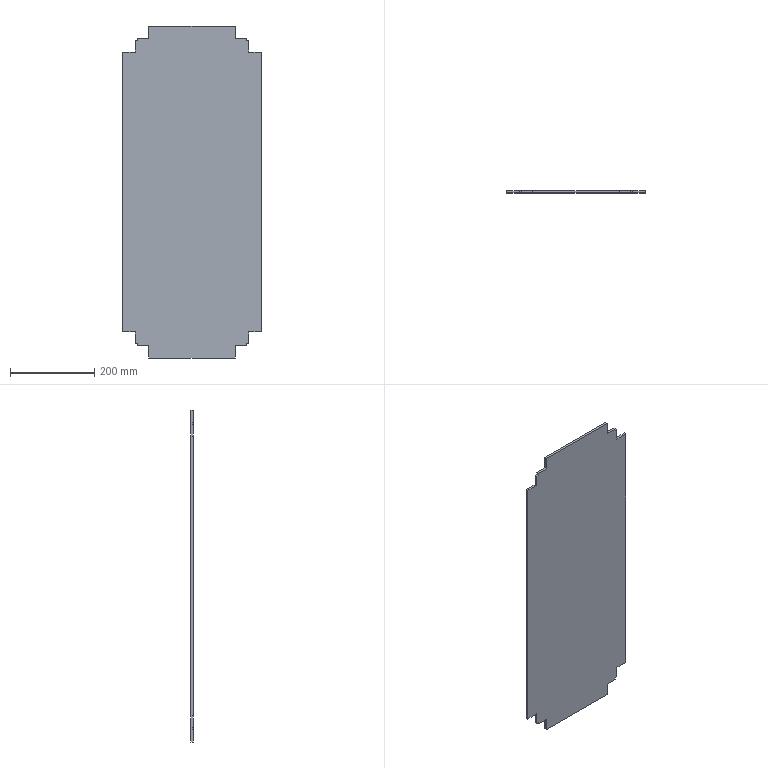Part | SolidWorks | features BaseBody 1 | 1 solid | 30 faces | box 330 x 5 x 790 mm | volume 1246600 mm3 | plane 30
STEP:
#1=CARTESIAN_POINT('',(-833.,40.,-365.));
#2=VERTEX_POINT('',#1);
#3=CARTESIAN_POINT('',(-860.,40.,-365.));
#4=VERTEX_POINT('',#3);
#5=CARTESIAN_POINT('',(-833.,40.,-365.));
#6=DIRECTION('',(-1.,0.,0.));
#7=VECTOR('',#6,1000.);
#8=LINE('',#5,#7);
#9=EDGE_CURVE('',#2,#4,#8,.T.);
#10=ORIENTED_EDGE('',*,*,#9,.F.);
#11=CARTESIAN_POINT('',(-833.,40.,-395.));
#12=VERTEX_POINT('',#11);
#13=CARTESIAN_POINT('',(-833.,40.,-395.));
#14=DIRECTION('',(0.,0.,1.));
#15=VECTOR('',#14,1000.);
#16=LINE('',#13,#15);
#17=EDGE_CURVE('',#12,#2,#16,.T.);
#18=ORIENTED_EDGE('',*,*,#17,.F.);
#19=CARTESIAN_POINT('',(-627.,40.,-395.));
#20=VERTEX_POINT('',#19);
#21=CARTESIAN_POINT('',(-627.,40.,-395.));
#22=DIRECTION('',(-1.,0.,0.));
#23=VECTOR('',#22,1000.);
#24=LINE('',#21,#23);
#25=EDGE_CURVE('',#20,#12,#24,.T.);
#26=ORIENTED_EDGE('',*,*,#25,.F.);
#27=CARTESIAN_POINT('',(-627.,40.,-365.));
#28=VERTEX_POINT('',#27);
#29=CARTESIAN_POINT('',(-627.,40.,-365.));
#30=DIRECTION('',(0.,0.,-1.));
#31=VECTOR('',#30,1000.);
#32=LINE('',#29,#31);
#33=EDGE_CURVE('',#28,#20,#32,.T.);
#34=ORIENTED_EDGE('',*,*,#33,.F.);
#35=CARTESIAN_POINT('',(-600.,40.,-365.));
#36=VERTEX_POINT('',#35);
#37=CARTESIAN_POINT('',(-600.,40.,-365.));
#38=DIRECTION('',(-1.,0.,0.));
#39=VECTOR('',#38,1000.);
#40=LINE('',#37,#39);
#41=EDGE_CURVE('',#36,#28,#40,.T.);
#42=ORIENTED_EDGE('',*,*,#41,.F.);
#43=CARTESIAN_POINT('',(-600.,40.,-360.));
#44=VERTEX_POINT('',#43);
#45=CARTESIAN_POINT('',(-600.,40.,-360.));
#46=DIRECTION('',(0.,0.,-1.));
#47=VECTOR('',#46,1000.);
#48=LINE('',#45,#47);
#49=EDGE_CURVE('',#44,#36,#48,.T.);
#50=ORIENTED_EDGE('',*,*,#49,.F.);
#51=CARTESIAN_POINT('',(-595.,40.,-360.));
#52=VERTEX_POINT('',#51);
#53=CARTESIAN_POINT('',(-595.,40.,-360.));
#54=DIRECTION('',(-1.,0.,0.));
#55=VECTOR('',#54,1000.);
#56=LINE('',#53,#55);
#57=EDGE_CURVE('',#52,#44,#56,.T.);
#58=ORIENTED_EDGE('',*,*,#57,.F.);
#59=CARTESIAN_POINT('',(-595.,40.,-333.));
#60=VERTEX_POINT('',#59);
#61=CARTESIAN_POINT('',(-595.,40.,-333.));
#62=DIRECTION('',(0.,0.,-1.));
#63=VECTOR('',#62,1000.);
#64=LINE('',#61,#63);
#65=EDGE_CURVE('',#60,#52,#64,.T.);
#66=ORIENTED_EDGE('',*,*,#65,.F.);
#67=CARTESIAN_POINT('',(-565.,40.,-333.));
#68=VERTEX_POINT('',#67);
#69=CARTESIAN_POINT('',(-565.,40.,-333.));
#70=DIRECTION('',(-1.,0.,0.));
#71=VECTOR('',#70,1000.);
#72=LINE('',#69,#71);
#73=EDGE_CURVE('',#68,#60,#72,.T.);
#74=ORIENTED_EDGE('',*,*,#73,.F.);
#75=CARTESIAN_POINT('',(-565.,40.,333.));
#76=VERTEX_POINT('',#75);
#77=CARTESIAN_POINT('',(-565.,40.,333.));
#78=DIRECTION('',(0.,0.,-1.));
#79=VECTOR('',#78,1000.);
#80=LINE('',#77,#79);
#81=EDGE_CURVE('',#76,#68,#80,.T.);
#82=ORIENTED_EDGE('',*,*,#81,.F.);
#83=CARTESIAN_POINT('',(-595.,40.,333.));
#84=VERTEX_POINT('',#83);
#85=CARTESIAN_POINT('',(-595.,40.,333.));
#86=DIRECTION('',(1.,0.,0.));
#87=VECTOR('',#86,1000.);
#88=LINE('',#85,#87);
#89=EDGE_CURVE('',#84,#76,#88,.T.);
#90=ORIENTED_EDGE('',*,*,#89,.F.);
#91=CARTESIAN_POINT('',(-595.,40.,360.));
#92=VERTEX_POINT('',#91);
#93=CARTESIAN_POINT('',(-595.,40.,360.));
#94=DIRECTION('',(0.,0.,-1.));
#95=VECTOR('',#94,1000.);
#96=LINE('',#93,#95);
#97=EDGE_CURVE('',#92,#84,#96,.T.);
#98=ORIENTED_EDGE('',*,*,#97,.F.);
#99=CARTESIAN_POINT('',(-600.,40.,360.));
#100=VERTEX_POINT('',#99);
#101=CARTESIAN_POINT('',(-600.,40.,360.));
#102=DIRECTION('',(1.,0.,0.));
#103=VECTOR('',#102,1000.);
#104=LINE('',#101,#103);
#105=EDGE_CURVE('',#100,#92,#104,.T.);
#106=ORIENTED_EDGE('',*,*,#105,.F.);
#107=CARTESIAN_POINT('',(-600.,40.,365.));
#108=VERTEX_POINT('',#107);
#109=CARTESIAN_POINT('',(-600.,40.,365.));
#110=DIRECTION('',(0.,0.,-1.));
#111=VECTOR('',#110,1000.);
#112=LINE('',#109,#111);
#113=EDGE_CURVE('',#108,#100,#112,.T.);
#114=ORIENTED_EDGE('',*,*,#113,.F.);
#115=CARTESIAN_POINT('',(-627.,40.,365.));
#116=VERTEX_POINT('',#115);
#117=CARTESIAN_POINT('',(-627.,40.,365.));
#118=DIRECTION('',(1.,0.,0.));
#119=VECTOR('',#118,1000.);
#120=LINE('',#117,#119);
#121=EDGE_CURVE('',#116,#108,#120,.T.);
#122=ORIENTED_EDGE('',*,*,#121,.F.);
#123=CARTESIAN_POINT('',(-627.,40.,395.));
#124=VERTEX_POINT('',#123);
#125=CARTESIAN_POINT('',(-627.,40.,395.));
#126=DIRECTION('',(0.,0.,-1.));
#127=VECTOR('',#126,1000.);
#128=LINE('',#125,#127);
#129=EDGE_CURVE('',#124,#116,#128,.T.);
#130=ORIENTED_EDGE('',*,*,#129,.F.);
#131=CARTESIAN_POINT('',(-833.,40.,395.));
#132=VERTEX_POINT('',#131);
#133=CARTESIAN_POINT('',(-833.,40.,395.));
#134=DIRECTION('',(1.,0.,0.));
#135=VECTOR('',#134,1000.);
#136=LINE('',#133,#135);
#137=EDGE_CURVE('',#132,#124,#136,.T.);
#138=ORIENTED_EDGE('',*,*,#137,.F.);
#139=CARTESIAN_POINT('',(-833.,40.,365.));
#140=VERTEX_POINT('',#139);
#141=CARTESIAN_POINT('',(-833.,40.,365.));
#142=DIRECTION('',(0.,0.,1.));
#143=VECTOR('',#142,1000.);
#144=LINE('',#141,#143);
#145=EDGE_CURVE('',#140,#132,#144,.T.);
#146=ORIENTED_EDGE('',*,*,#145,.F.);
#147=CARTESIAN_POINT('',(-860.,40.,365.));
#148=VERTEX_POINT('',#147);
#149=CARTESIAN_POINT('',(-860.,40.,365.));
#150=DIRECTION('',(1.,0.,0.));
#151=VECTOR('',#150,1000.);
#152=LINE('',#149,#151);
#153=EDGE_CURVE('',#148,#140,#152,.T.);
#154=ORIENTED_EDGE('',*,*,#153,.F.);
#155=CARTESIAN_POINT('',(-860.,40.,360.));
#156=VERTEX_POINT('',#155);
#157=CARTESIAN_POINT('',(-860.,40.,360.));
#158=DIRECTION('',(0.,0.,1.));
#159=VECTOR('',#158,1000.);
#160=LINE('',#157,#159);
#161=EDGE_CURVE('',#156,#148,#160,.T.);
#162=ORIENTED_EDGE('',*,*,#161,.F.);
#163=CARTESIAN_POINT('',(-865.,40.,360.));
#164=VERTEX_POINT('',#163);
#165=CARTESIAN_POINT('',(-865.,40.,360.));
#166=DIRECTION('',(1.,0.,0.));
#167=VECTOR('',#166,1000.);
#168=LINE('',#165,#167);
#169=EDGE_CURVE('',#164,#156,#168,.T.);
#170=ORIENTED_EDGE('',*,*,#169,.F.);
#171=CARTESIAN_POINT('',(-865.,40.,333.));
#172=VERTEX_POINT('',#171);
#173=CARTESIAN_POINT('',(-865.,40.,333.));
#174=DIRECTION('',(0.,0.,1.));
#175=VECTOR('',#174,1000.);
#176=LINE('',#173,#175);
#177=EDGE_CURVE('',#172,#164,#176,.T.);
#178=ORIENTED_EDGE('',*,*,#177,.F.);
#179=CARTESIAN_POINT('',(-895.,40.,333.));
#180=VERTEX_POINT('',#179);
#181=CARTESIAN_POINT('',(-895.,40.,333.));
#182=DIRECTION('',(1.,0.,0.));
#183=VECTOR('',#182,1000.);
#184=LINE('',#181,#183);
#185=EDGE_CURVE('',#180,#172,#184,.T.);
#186=ORIENTED_EDGE('',*,*,#185,.F.);
#187=CARTESIAN_POINT('',(-895.,40.,-333.));
#188=VERTEX_POINT('',#187);
#189=CARTESIAN_POINT('',(-895.,40.,-333.));
#190=DIRECTION('',(0.,0.,1.));
#191=VECTOR('',#190,1000.);
#192=LINE('',#189,#191);
#193=EDGE_CURVE('',#188,#180,#192,.T.);
#194=ORIENTED_EDGE('',*,*,#193,.F.);
#195=CARTESIAN_POINT('',(-865.,40.,-333.));
#196=VERTEX_POINT('',#195);
#197=CARTESIAN_POINT('',(-865.,40.,-333.));
#198=DIRECTION('',(-1.,0.,0.));
#199=VECTOR('',#198,1000.);
#200=LINE('',#197,#199);
#201=EDGE_CURVE('',#196,#188,#200,.T.);
#202=ORIENTED_EDGE('',*,*,#201,.F.);
#203=CARTESIAN_POINT('',(-865.,40.,-360.));
#204=VERTEX_POINT('',#203);
#205=CARTESIAN_POINT('',(-865.,40.,-360.));
#206=DIRECTION('',(0.,0.,1.));
#207=VECTOR('',#206,1000.);
#208=LINE('',#205,#207);
#209=EDGE_CURVE('',#204,#196,#208,.T.);
#210=ORIENTED_EDGE('',*,*,#209,.F.);
#211=CARTESIAN_POINT('',(-860.,40.,-360.));
#212=VERTEX_POINT('',#211);
#213=CARTESIAN_POINT('',(-860.,40.,-360.));
#214=DIRECTION('',(-1.,0.,0.));
#215=VECTOR('',#214,1000.);
#216=LINE('',#213,#215);
#217=EDGE_CURVE('',#212,#204,#216,.T.);
#218=ORIENTED_EDGE('',*,*,#217,.F.);
#219=CARTESIAN_POINT('',(-860.,40.,-365.));
#220=DIRECTION('',(0.,0.,1.));
#221=VECTOR('',#220,1000.);
#222=LINE('',#219,#221);
#223=EDGE_CURVE('',#4,#212,#222,.T.);
#224=ORIENTED_EDGE('',*,*,#223,.F.);
#225=EDGE_LOOP('',(#10,#18,#26,#34,#42,#50,#58,#66,#74,#82,#90,#98,#106,#114,#122,#130,#138,#146,#154,#162,#170,#178,#186,#194,#202,#210,#218,#224));
#226=FACE_OUTER_BOUND('',#225,.T.);
#227=CARTESIAN_POINT('',(-730.,40.,0.));
#228=DIRECTION('',(0.,-1.,0.));
#229=DIRECTION('',(0.,0.,-1.));
#230=AXIS2_PLACEMENT_3D('',#227,#228,#229);
#231=PLANE('',#230);
#232=ADVANCED_FACE('',(#226),#231,.T.);
#233=CARTESIAN_POINT('',(-860.,45.,-365.));
#234=VERTEX_POINT('',#233);
#235=CARTESIAN_POINT('',(-833.,45.,-365.));
#236=VERTEX_POINT('',#235);
#237=CARTESIAN_POINT('',(-860.,45.,-365.));
#238=DIRECTION('',(1.,0.,0.));
#239=VECTOR('',#238,1000.);
#240=LINE('',#237,#239);
#241=EDGE_CURVE('',#234,#236,#240,.T.);
#242=ORIENTED_EDGE('',*,*,#241,.F.);
#243=CARTESIAN_POINT('',(-860.,45.,-360.));
#244=VERTEX_POINT('',#243);
#245=CARTESIAN_POINT('',(-860.,45.,-360.));
#246=DIRECTION('',(0.,0.,-1.));
#247=VECTOR('',#246,1000.);
#248=LINE('',#245,#247);
#249=EDGE_CURVE('',#244,#234,#248,.T.);
#250=ORIENTED_EDGE('',*,*,#249,.F.);
#251=CARTESIAN_POINT('',(-865.,45.,-360.));
#252=VERTEX_POINT('',#251);
#253=CARTESIAN_POINT('',(-865.,45.,-360.));
#254=DIRECTION('',(1.,0.,0.));
#255=VECTOR('',#254,1000.);
#256=LINE('',#253,#255);
#257=EDGE_CURVE('',#252,#244,#256,.T.);
#258=ORIENTED_EDGE('',*,*,#257,.F.);
#259=CARTESIAN_POINT('',(-865.,45.,-333.));
#260=VERTEX_POINT('',#259);
#261=CARTESIAN_POINT('',(-865.,45.,-333.));
#262=DIRECTION('',(0.,0.,-1.));
#263=VECTOR('',#262,1000.);
#264=LINE('',#261,#263);
#265=EDGE_CURVE('',#260,#252,#264,.T.);
#266=ORIENTED_EDGE('',*,*,#265,.F.);
#267=CARTESIAN_POINT('',(-895.,45.,-333.));
#268=VERTEX_POINT('',#267);
#269=CARTESIAN_POINT('',(-895.,45.,-333.));
#270=DIRECTION('',(1.,0.,0.));
#271=VECTOR('',#270,1000.);
#272=LINE('',#269,#271);
#273=EDGE_CURVE('',#268,#260,#272,.T.);
#274=ORIENTED_EDGE('',*,*,#273,.F.);
#275=CARTESIAN_POINT('',(-895.,45.,333.));
#276=VERTEX_POINT('',#275);
#277=CARTESIAN_POINT('',(-895.,45.,333.));
#278=DIRECTION('',(0.,0.,-1.));
#279=VECTOR('',#278,1000.);
#280=LINE('',#277,#279);
#281=EDGE_CURVE('',#276,#268,#280,.T.);
#282=ORIENTED_EDGE('',*,*,#281,.F.);
#283=CARTESIAN_POINT('',(-865.,45.,333.));
#284=VERTEX_POINT('',#283);
#285=CARTESIAN_POINT('',(-865.,45.,333.));
#286=DIRECTION('',(-1.,0.,0.));
#287=VECTOR('',#286,1000.);
#288=LINE('',#285,#287);
#289=EDGE_CURVE('',#284,#276,#288,.T.);
#290=ORIENTED_EDGE('',*,*,#289,.F.);
#291=CARTESIAN_POINT('',(-865.,45.,360.));
#292=VERTEX_POINT('',#291);
#293=CARTESIAN_POINT('',(-865.,45.,360.));
#294=DIRECTION('',(0.,0.,-1.));
#295=VECTOR('',#294,1000.);
#296=LINE('',#293,#295);
#297=EDGE_CURVE('',#292,#284,#296,.T.);
#298=ORIENTED_EDGE('',*,*,#297,.F.);
#299=CARTESIAN_POINT('',(-860.,45.,360.));
#300=VERTEX_POINT('',#299);
#301=CARTESIAN_POINT('',(-860.,45.,360.));
#302=DIRECTION('',(-1.,0.,0.));
#303=VECTOR('',#302,1000.);
#304=LINE('',#301,#303);
#305=EDGE_CURVE('',#300,#292,#304,.T.);
#306=ORIENTED_EDGE('',*,*,#305,.F.);
#307=CARTESIAN_POINT('',(-860.,45.,365.));
#308=VERTEX_POINT('',#307);
#309=CARTESIAN_POINT('',(-860.,45.,365.));
#310=DIRECTION('',(0.,0.,-1.));
#311=VECTOR('',#310,1000.);
#312=LINE('',#309,#311);
#313=EDGE_CURVE('',#308,#300,#312,.T.);
#314=ORIENTED_EDGE('',*,*,#313,.F.);
#315=CARTESIAN_POINT('',(-833.,45.,365.));
#316=VERTEX_POINT('',#315);
#317=CARTESIAN_POINT('',(-833.,45.,365.));
#318=DIRECTION('',(-1.,0.,0.));
#319=VECTOR('',#318,1000.);
#320=LINE('',#317,#319);
#321=EDGE_CURVE('',#316,#308,#320,.T.);
#322=ORIENTED_EDGE('',*,*,#321,.F.);
#323=CARTESIAN_POINT('',(-833.,45.,395.));
#324=VERTEX_POINT('',#323);
#325=CARTESIAN_POINT('',(-833.,45.,395.));
#326=DIRECTION('',(0.,0.,-1.));
#327=VECTOR('',#326,1000.);
#328=LINE('',#325,#327);
#329=EDGE_CURVE('',#324,#316,#328,.T.);
#330=ORIENTED_EDGE('',*,*,#329,.F.);
#331=CARTESIAN_POINT('',(-627.,45.,395.));
#332=VERTEX_POINT('',#331);
#333=CARTESIAN_POINT('',(-627.,45.,395.));
#334=DIRECTION('',(-1.,0.,0.));
#335=VECTOR('',#334,1000.);
#336=LINE('',#333,#335);
#337=EDGE_CURVE('',#332,#324,#336,.T.);
#338=ORIENTED_EDGE('',*,*,#337,.F.);
#339=CARTESIAN_POINT('',(-627.,45.,365.));
#340=VERTEX_POINT('',#339);
#341=CARTESIAN_POINT('',(-627.,45.,365.));
#342=DIRECTION('',(0.,0.,1.));
#343=VECTOR('',#342,1000.);
#344=LINE('',#341,#343);
#345=EDGE_CURVE('',#340,#332,#344,.T.);
#346=ORIENTED_EDGE('',*,*,#345,.F.);
#347=CARTESIAN_POINT('',(-600.,45.,365.));
#348=VERTEX_POINT('',#347);
#349=CARTESIAN_POINT('',(-600.,45.,365.));
#350=DIRECTION('',(-1.,0.,0.));
#351=VECTOR('',#350,1000.);
#352=LINE('',#349,#351);
#353=EDGE_CURVE('',#348,#340,#352,.T.);
#354=ORIENTED_EDGE('',*,*,#353,.F.);
#355=CARTESIAN_POINT('',(-600.,45.,360.));
#356=VERTEX_POINT('',#355);
#357=CARTESIAN_POINT('',(-600.,45.,360.));
#358=DIRECTION('',(0.,0.,1.));
#359=VECTOR('',#358,1000.);
#360=LINE('',#357,#359);
#361=EDGE_CURVE('',#356,#348,#360,.T.);
#362=ORIENTED_EDGE('',*,*,#361,.F.);
#363=CARTESIAN_POINT('',(-595.,45.,360.));
#364=VERTEX_POINT('',#363);
#365=CARTESIAN_POINT('',(-595.,45.,360.));
#366=DIRECTION('',(-1.,0.,0.));
#367=VECTOR('',#366,1000.);
#368=LINE('',#365,#367);
#369=EDGE_CURVE('',#364,#356,#368,.T.);
#370=ORIENTED_EDGE('',*,*,#369,.F.);
#371=CARTESIAN_POINT('',(-595.,45.,333.));
#372=VERTEX_POINT('',#371);
#373=CARTESIAN_POINT('',(-595.,45.,333.));
#374=DIRECTION('',(0.,0.,1.));
#375=VECTOR('',#374,1000.);
#376=LINE('',#373,#375);
#377=EDGE_CURVE('',#372,#364,#376,.T.);
#378=ORIENTED_EDGE('',*,*,#377,.F.);
#379=CARTESIAN_POINT('',(-565.,45.,333.));
#380=VERTEX_POINT('',#379);
#381=CARTESIAN_POINT('',(-565.,45.,333.));
#382=DIRECTION('',(-1.,0.,0.));
#383=VECTOR('',#382,1000.);
#384=LINE('',#381,#383);
#385=EDGE_CURVE('',#380,#372,#384,.T.);
#386=ORIENTED_EDGE('',*,*,#385,.F.);
#387=CARTESIAN_POINT('',(-565.,45.,-333.));
#388=VERTEX_POINT('',#387);
#389=CARTESIAN_POINT('',(-565.,45.,-333.));
#390=DIRECTION('',(0.,0.,1.));
#391=VECTOR('',#390,1000.);
#392=LINE('',#389,#391);
#393=EDGE_CURVE('',#388,#380,#392,.T.);
#394=ORIENTED_EDGE('',*,*,#393,.F.);
#395=CARTESIAN_POINT('',(-595.,45.,-333.));
#396=VERTEX_POINT('',#395);
#397=CARTESIAN_POINT('',(-595.,45.,-333.));
#398=DIRECTION('',(1.,0.,0.));
#399=VECTOR('',#398,1000.);
#400=LINE('',#397,#399);
#401=EDGE_CURVE('',#396,#388,#400,.T.);
#402=ORIENTED_EDGE('',*,*,#401,.F.);
#403=CARTESIAN_POINT('',(-595.,45.,-360.));
#404=VERTEX_POINT('',#403);
#405=CARTESIAN_POINT('',(-595.,45.,-360.));
#406=DIRECTION('',(0.,0.,1.));
#407=VECTOR('',#406,1000.);
#408=LINE('',#405,#407);
#409=EDGE_CURVE('',#404,#396,#408,.T.);
#410=ORIENTED_EDGE('',*,*,#409,.F.);
#411=CARTESIAN_POINT('',(-600.,45.,-360.));
#412=VERTEX_POINT('',#411);
#413=CARTESIAN_POINT('',(-600.,45.,-360.));
#414=DIRECTION('',(1.,0.,0.));
#415=VECTOR('',#414,1000.);
#416=LINE('',#413,#415);
#417=EDGE_CURVE('',#412,#404,#416,.T.);
#418=ORIENTED_EDGE('',*,*,#417,.F.);
#419=CARTESIAN_POINT('',(-600.,45.,-365.));
#420=VERTEX_POINT('',#419);
#421=CARTESIAN_POINT('',(-600.,45.,-365.));
#422=DIRECTION('',(0.,0.,1.));
#423=VECTOR('',#422,1000.);
#424=LINE('',#421,#423);
#425=EDGE_CURVE('',#420,#412,#424,.T.);
#426=ORIENTED_EDGE('',*,*,#425,.F.);
#427=CARTESIAN_POINT('',(-627.,45.,-365.));
#428=VERTEX_POINT('',#427);
#429=CARTESIAN_POINT('',(-627.,45.,-365.));
#430=DIRECTION('',(1.,0.,0.));
#431=VECTOR('',#430,1000.);
#432=LINE('',#429,#431);
#433=EDGE_CURVE('',#428,#420,#432,.T.);
#434=ORIENTED_EDGE('',*,*,#433,.F.);
#435=CARTESIAN_POINT('',(-627.,45.,-395.));
#436=VERTEX_POINT('',#435);
#437=CARTESIAN_POINT('',(-627.,45.,-395.));
#438=DIRECTION('',(0.,0.,1.));
#439=VECTOR('',#438,1000.);
#440=LINE('',#437,#439);
#441=EDGE_CURVE('',#436,#428,#440,.T.);
#442=ORIENTED_EDGE('',*,*,#441,.F.);
#443=CARTESIAN_POINT('',(-833.,45.,-395.));
#444=VERTEX_POINT('',#443);
#445=CARTESIAN_POINT('',(-833.,45.,-395.));
#446=DIRECTION('',(1.,0.,0.));
#447=VECTOR('',#446,1000.);
#448=LINE('',#445,#447);
#449=EDGE_CURVE('',#444,#436,#448,.T.);
#450=ORIENTED_EDGE('',*,*,#449,.F.);
#451=CARTESIAN_POINT('',(-833.,45.,-365.));
#452=DIRECTION('',(0.,0.,-1.));
#453=VECTOR('',#452,1000.);
#454=LINE('',#451,#453);
#455=EDGE_CURVE('',#236,#444,#454,.T.);
#456=ORIENTED_EDGE('',*,*,#455,.F.);
#457=EDGE_LOOP('',(#242,#250,#258,#266,#274,#282,#290,#298,#306,#314,#322,#330,#338,#346,#354,#362,#370,#378,#386,#394,#402,#410,#418,#426,#434,#442,#450,#456));
#458=FACE_OUTER_BOUND('',#457,.T.);
#459=CARTESIAN_POINT('',(-730.,45.,0.));
#460=DIRECTION('',(0.,1.,0.));
#461=DIRECTION('',(1.,0.,0.));
#462=AXIS2_PLACEMENT_3D('',#459,#460,#461);
#463=PLANE('',#462);
#464=ADVANCED_FACE('',(#458),#463,.T.);
#465=ORIENTED_EDGE('',*,*,#9,.T.);
#466=CARTESIAN_POINT('',(-860.,45.,-365.));
#467=DIRECTION('',(0.,-1.,0.));
#468=VECTOR('',#467,1000.);
#469=LINE('',#466,#468);
#470=EDGE_CURVE('',#234,#4,#469,.T.);
#471=ORIENTED_EDGE('',*,*,#470,.F.);
#472=ORIENTED_EDGE('',*,*,#241,.T.);
#473=CARTESIAN_POINT('',(-833.,40.,-365.));
#474=DIRECTION('',(0.,1.,0.));
#475=VECTOR('',#474,1000.);
#476=LINE('',#473,#475);
#477=EDGE_CURVE('',#2,#236,#476,.T.);
#478=ORIENTED_EDGE('',*,*,#477,.F.);
#479=EDGE_LOOP('',(#465,#471,#472,#478));
#480=FACE_OUTER_BOUND('',#479,.T.);
#481=CARTESIAN_POINT('',(-833.,40.,-365.));
#482=DIRECTION('',(0.,0.,-1.));
#483=DIRECTION('',(0.,-1.,0.));
#484=AXIS2_PLACEMENT_3D('',#481,#482,#483);
#485=PLANE('',#484);
#486=ADVANCED_FACE('',(#480),#485,.T.);
#487=ORIENTED_EDGE('',*,*,#223,.T.);
#488=CARTESIAN_POINT('',(-860.,45.,-360.));
#489=DIRECTION('',(0.,-1.,0.));
#490=VECTOR('',#489,1000.);
#491=LINE('',#488,#490);
#492=EDGE_CURVE('',#244,#212,#491,.T.);
#493=ORIENTED_EDGE('',*,*,#492,.F.);
#494=ORIENTED_EDGE('',*,*,#249,.T.);
#495=ORIENTED_EDGE('',*,*,#470,.T.);
#496=EDGE_LOOP('',(#487,#493,#494,#495));
#497=FACE_OUTER_BOUND('',#496,.T.);
#498=CARTESIAN_POINT('',(-860.,40.,-365.));
#499=DIRECTION('',(-1.,0.,0.));
#500=DIRECTION('',(0.,0.,1.));
#501=AXIS2_PLACEMENT_3D('',#498,#499,#500);
#502=PLANE('',#501);
#503=ADVANCED_FACE('',(#497),#502,.T.);
#504=ORIENTED_EDGE('',*,*,#217,.T.);
#505=CARTESIAN_POINT('',(-865.,45.,-360.));
#506=DIRECTION('',(0.,-1.,0.));
#507=VECTOR('',#506,1000.);
#508=LINE('',#505,#507);
#509=EDGE_CURVE('',#252,#204,#508,.T.);
#510=ORIENTED_EDGE('',*,*,#509,.F.);
#511=ORIENTED_EDGE('',*,*,#257,.T.);
#512=ORIENTED_EDGE('',*,*,#492,.T.);
#513=EDGE_LOOP('',(#504,#510,#511,#512));
#514=FACE_OUTER_BOUND('',#513,.T.);
#515=CARTESIAN_POINT('',(-860.,40.,-360.));
#516=DIRECTION('',(0.,0.,-1.));
#517=DIRECTION('',(0.,-1.,0.));
#518=AXIS2_PLACEMENT_3D('',#515,#516,#517);
#519=PLANE('',#518);
#520=ADVANCED_FACE('',(#514),#519,.T.);
#521=ORIENTED_EDGE('',*,*,#209,.T.);
#522=CARTESIAN_POINT('',(-865.,45.,-333.));
#523=DIRECTION('',(0.,-1.,0.));
#524=VECTOR('',#523,1000.);
#525=LINE('',#522,#524);
#526=EDGE_CURVE('',#260,#196,#525,.T.);
#527=ORIENTED_EDGE('',*,*,#526,.F.);
#528=ORIENTED_EDGE('',*,*,#265,.T.);
#529=ORIENTED_EDGE('',*,*,#509,.T.);
#530=EDGE_LOOP('',(#521,#527,#528,#529));
#531=FACE_OUTER_BOUND('',#530,.T.);
#532=CARTESIAN_POINT('',(-865.,40.,-360.));
#533=DIRECTION('',(-1.,0.,0.));
#534=DIRECTION('',(0.,0.,1.));
#535=AXIS2_PLACEMENT_3D('',#532,#533,#534);
#536=PLANE('',#535);
#537=ADVANCED_FACE('',(#531),#536,.T.);
#538=ORIENTED_EDGE('',*,*,#201,.T.);
#539=CARTESIAN_POINT('',(-895.,45.,-333.));
#540=DIRECTION('',(0.,-1.,0.));
#541=VECTOR('',#540,1000.);
#542=LINE('',#539,#541);
#543=EDGE_CURVE('',#268,#188,#542,.T.);
#544=ORIENTED_EDGE('',*,*,#543,.F.);
#545=ORIENTED_EDGE('',*,*,#273,.T.);
#546=ORIENTED_EDGE('',*,*,#526,.T.);
#547=EDGE_LOOP('',(#538,#544,#545,#546));
#548=FACE_OUTER_BOUND('',#547,.T.);
#549=CARTESIAN_POINT('',(-865.,40.,-333.));
#550=DIRECTION('',(0.,0.,-1.));
#551=DIRECTION('',(0.,-1.,0.));
#552=AXIS2_PLACEMENT_3D('',#549,#550,#551);
#553=PLANE('',#552);
#554=ADVANCED_FACE('',(#548),#553,.T.);
#555=ORIENTED_EDGE('',*,*,#193,.T.);
#556=CARTESIAN_POINT('',(-895.,45.,333.));
#557=DIRECTION('',(0.,-1.,0.));
#558=VECTOR('',#557,1000.);
#559=LINE('',#556,#558);
#560=EDGE_CURVE('',#276,#180,#559,.T.);
#561=ORIENTED_EDGE('',*,*,#560,.F.);
#562=ORIENTED_EDGE('',*,*,#281,.T.);
#563=ORIENTED_EDGE('',*,*,#543,.T.);
#564=EDGE_LOOP('',(#555,#561,#562,#563));
#565=FACE_OUTER_BOUND('',#564,.T.);
#566=CARTESIAN_POINT('',(-895.,40.,-333.));
#567=DIRECTION('',(-1.,0.,0.));
#568=DIRECTION('',(0.,0.,1.));
#569=AXIS2_PLACEMENT_3D('',#566,#567,#568);
#570=PLANE('',#569);
#571=ADVANCED_FACE('',(#565),#570,.T.);
#572=ORIENTED_EDGE('',*,*,#185,.T.);
#573=CARTESIAN_POINT('',(-865.,45.,333.));
#574=DIRECTION('',(0.,-1.,0.));
#575=VECTOR('',#574,1000.);
#576=LINE('',#573,#575);
#577=EDGE_CURVE('',#284,#172,#576,.T.);
#578=ORIENTED_EDGE('',*,*,#577,.F.);
#579=ORIENTED_EDGE('',*,*,#289,.T.);
#580=ORIENTED_EDGE('',*,*,#560,.T.);
#581=EDGE_LOOP('',(#572,#578,#579,#580));
#582=FACE_OUTER_BOUND('',#581,.T.);
#583=CARTESIAN_POINT('',(-895.,40.,333.));
#584=DIRECTION('',(0.,0.,1.));
#585=DIRECTION('',(1.,0.,0.));
#586=AXIS2_PLACEMENT_3D('',#583,#584,#585);
#587=PLANE('',#586);
#588=ADVANCED_FACE('',(#582),#587,.T.);
#589=ORIENTED_EDGE('',*,*,#177,.T.);
#590=CARTESIAN_POINT('',(-865.,45.,360.));
#591=DIRECTION('',(0.,-1.,0.));
#592=VECTOR('',#591,1000.);
#593=LINE('',#590,#592);
#594=EDGE_CURVE('',#292,#164,#593,.T.);
#595=ORIENTED_EDGE('',*,*,#594,.F.);
#596=ORIENTED_EDGE('',*,*,#297,.T.);
#597=ORIENTED_EDGE('',*,*,#577,.T.);
#598=EDGE_LOOP('',(#589,#595,#596,#597));
#599=FACE_OUTER_BOUND('',#598,.T.);
#600=CARTESIAN_POINT('',(-865.,40.,333.));
#601=DIRECTION('',(-1.,0.,0.));
#602=DIRECTION('',(0.,0.,1.));
#603=AXIS2_PLACEMENT_3D('',#600,#601,#602);
#604=PLANE('',#603);
#605=ADVANCED_FACE('',(#599),#604,.T.);
#606=ORIENTED_EDGE('',*,*,#169,.T.);
#607=CARTESIAN_POINT('',(-860.,45.,360.));
#608=DIRECTION('',(0.,-1.,0.));
#609=VECTOR('',#608,1000.);
#610=LINE('',#607,#609);
#611=EDGE_CURVE('',#300,#156,#610,.T.);
#612=ORIENTED_EDGE('',*,*,#611,.F.);
#613=ORIENTED_EDGE('',*,*,#305,.T.);
#614=ORIENTED_EDGE('',*,*,#594,.T.);
#615=EDGE_LOOP('',(#606,#612,#613,#614));
#616=FACE_OUTER_BOUND('',#615,.T.);
#617=CARTESIAN_POINT('',(-865.,40.,360.));
#618=DIRECTION('',(0.,0.,1.));
#619=DIRECTION('',(1.,0.,0.));
#620=AXIS2_PLACEMENT_3D('',#617,#618,#619);
#621=PLANE('',#620);
#622=ADVANCED_FACE('',(#616),#621,.T.);
#623=ORIENTED_EDGE('',*,*,#161,.T.);
#624=CARTESIAN_POINT('',(-860.,45.,365.));
#625=DIRECTION('',(0.,-1.,0.));
#626=VECTOR('',#625,1000.);
#627=LINE('',#624,#626);
#628=EDGE_CURVE('',#308,#148,#627,.T.);
#629=ORIENTED_EDGE('',*,*,#628,.F.);
#630=ORIENTED_EDGE('',*,*,#313,.T.);
#631=ORIENTED_EDGE('',*,*,#611,.T.);
#632=EDGE_LOOP('',(#623,#629,#630,#631));
#633=FACE_OUTER_BOUND('',#632,.T.);
#634=CARTESIAN_POINT('',(-860.,40.,360.));
#635=DIRECTION('',(-1.,0.,0.));
#636=DIRECTION('',(0.,0.,1.));
#637=AXIS2_PLACEMENT_3D('',#634,#635,#636);
#638=PLANE('',#637);
#639=ADVANCED_FACE('',(#633),#638,.T.);
#640=ORIENTED_EDGE('',*,*,#153,.T.);
#641=CARTESIAN_POINT('',(-833.,45.,365.));
#642=DIRECTION('',(0.,-1.,0.));
#643=VECTOR('',#642,1000.);
#644=LINE('',#641,#643);
#645=EDGE_CURVE('',#316,#140,#644,.T.);
#646=ORIENTED_EDGE('',*,*,#645,.F.);
#647=ORIENTED_EDGE('',*,*,#321,.T.);
#648=ORIENTED_EDGE('',*,*,#628,.T.);
#649=EDGE_LOOP('',(#640,#646,#647,#648));
#650=FACE_OUTER_BOUND('',#649,.T.);
#651=CARTESIAN_POINT('',(-860.,40.,365.));
#652=DIRECTION('',(0.,0.,1.));
#653=DIRECTION('',(1.,0.,0.));
#654=AXIS2_PLACEMENT_3D('',#651,#652,#653);
#655=PLANE('',#654);
#656=ADVANCED_FACE('',(#650),#655,.T.);
#657=ORIENTED_EDGE('',*,*,#145,.T.);
#658=CARTESIAN_POINT('',(-833.,45.,395.));
#659=DIRECTION('',(0.,-1.,0.));
#660=VECTOR('',#659,1000.);
#661=LINE('',#658,#660);
#662=EDGE_CURVE('',#324,#132,#661,.T.);
#663=ORIENTED_EDGE('',*,*,#662,.F.);
#664=ORIENTED_EDGE('',*,*,#329,.T.);
#665=ORIENTED_EDGE('',*,*,#645,.T.);
#666=EDGE_LOOP('',(#657,#663,#664,#665));
#667=FACE_OUTER_BOUND('',#666,.T.);
#668=CARTESIAN_POINT('',(-833.,40.,365.));
#669=DIRECTION('',(-1.,0.,0.));
#670=DIRECTION('',(0.,0.,1.));
#671=AXIS2_PLACEMENT_3D('',#668,#669,#670);
#672=PLANE('',#671);
#673=ADVANCED_FACE('',(#667),#672,.T.);
#674=ORIENTED_EDGE('',*,*,#137,.T.);
#675=CARTESIAN_POINT('',(-627.,45.,395.));
#676=DIRECTION('',(0.,-1.,0.));
#677=VECTOR('',#676,1000.);
#678=LINE('',#675,#677);
#679=EDGE_CURVE('',#332,#124,#678,.T.);
#680=ORIENTED_EDGE('',*,*,#679,.F.);
#681=ORIENTED_EDGE('',*,*,#337,.T.);
#682=ORIENTED_EDGE('',*,*,#662,.T.);
#683=EDGE_LOOP('',(#674,#680,#681,#682));
#684=FACE_OUTER_BOUND('',#683,.T.);
#685=CARTESIAN_POINT('',(-833.,40.,395.));
#686=DIRECTION('',(0.,0.,1.));
#687=DIRECTION('',(1.,0.,0.));
#688=AXIS2_PLACEMENT_3D('',#685,#686,#687);
#689=PLANE('',#688);
#690=ADVANCED_FACE('',(#684),#689,.T.);
#691=ORIENTED_EDGE('',*,*,#129,.T.);
#692=CARTESIAN_POINT('',(-627.,45.,365.));
#693=DIRECTION('',(0.,-1.,0.));
#694=VECTOR('',#693,1000.);
#695=LINE('',#692,#694);
#696=EDGE_CURVE('',#340,#116,#695,.T.);
#697=ORIENTED_EDGE('',*,*,#696,.F.);
#698=ORIENTED_EDGE('',*,*,#345,.T.);
#699=ORIENTED_EDGE('',*,*,#679,.T.);
#700=EDGE_LOOP('',(#691,#697,#698,#699));
#701=FACE_OUTER_BOUND('',#700,.T.);
#702=CARTESIAN_POINT('',(-627.,40.,395.));
#703=DIRECTION('',(1.,0.,0.));
#704=DIRECTION('',(0.,1.,0.));
#705=AXIS2_PLACEMENT_3D('',#702,#703,#704);
#706=PLANE('',#705);
#707=ADVANCED_FACE('',(#701),#706,.T.);
#708=ORIENTED_EDGE('',*,*,#121,.T.);
#709=CARTESIAN_POINT('',(-600.,45.,365.));
#710=DIRECTION('',(0.,-1.,0.));
#711=VECTOR('',#710,1000.);
#712=LINE('',#709,#711);
#713=EDGE_CURVE('',#348,#108,#712,.T.);
#714=ORIENTED_EDGE('',*,*,#713,.F.);
#715=ORIENTED_EDGE('',*,*,#353,.T.);
#716=ORIENTED_EDGE('',*,*,#696,.T.);
#717=EDGE_LOOP('',(#708,#714,#715,#716));
#718=FACE_OUTER_BOUND('',#717,.T.);
#719=CARTESIAN_POINT('',(-627.,40.,365.));
#720=DIRECTION('',(0.,0.,1.));
#721=DIRECTION('',(1.,0.,0.));
#722=AXIS2_PLACEMENT_3D('',#719,#720,#721);
#723=PLANE('',#722);
#724=ADVANCED_FACE('',(#718),#723,.T.);
#725=ORIENTED_EDGE('',*,*,#113,.T.);
#726=CARTESIAN_POINT('',(-600.,45.,360.));
#727=DIRECTION('',(0.,-1.,0.));
#728=VECTOR('',#727,1000.);
#729=LINE('',#726,#728);
#730=EDGE_CURVE('',#356,#100,#729,.T.);
#731=ORIENTED_EDGE('',*,*,#730,.F.);
#732=ORIENTED_EDGE('',*,*,#361,.T.);
#733=ORIENTED_EDGE('',*,*,#713,.T.);
#734=EDGE_LOOP('',(#725,#731,#732,#733));
#735=FACE_OUTER_BOUND('',#734,.T.);
#736=CARTESIAN_POINT('',(-600.,40.,365.));
#737=DIRECTION('',(1.,0.,0.));
#738=DIRECTION('',(0.,1.,0.));
#739=AXIS2_PLACEMENT_3D('',#736,#737,#738);
#740=PLANE('',#739);
#741=ADVANCED_FACE('',(#735),#740,.T.);
#742=ORIENTED_EDGE('',*,*,#105,.T.);
#743=CARTESIAN_POINT('',(-595.,45.,360.));
#744=DIRECTION('',(0.,-1.,0.));
#745=VECTOR('',#744,1000.);
#746=LINE('',#743,#745);
#747=EDGE_CURVE('',#364,#92,#746,.T.);
#748=ORIENTED_EDGE('',*,*,#747,.F.);
#749=ORIENTED_EDGE('',*,*,#369,.T.);
#750=ORIENTED_EDGE('',*,*,#730,.T.);
#751=EDGE_LOOP('',(#742,#748,#749,#750));
#752=FACE_OUTER_BOUND('',#751,.T.);
#753=CARTESIAN_POINT('',(-600.,40.,360.));
#754=DIRECTION('',(0.,0.,1.));
#755=DIRECTION('',(1.,0.,0.));
#756=AXIS2_PLACEMENT_3D('',#753,#754,#755);
#757=PLANE('',#756);
#758=ADVANCED_FACE('',(#752),#757,.T.);
#759=ORIENTED_EDGE('',*,*,#97,.T.);
#760=CARTESIAN_POINT('',(-595.,45.,333.));
#761=DIRECTION('',(0.,-1.,0.));
#762=VECTOR('',#761,1000.);
#763=LINE('',#760,#762);
#764=EDGE_CURVE('',#372,#84,#763,.T.);
#765=ORIENTED_EDGE('',*,*,#764,.F.);
#766=ORIENTED_EDGE('',*,*,#377,.T.);
#767=ORIENTED_EDGE('',*,*,#747,.T.);
#768=EDGE_LOOP('',(#759,#765,#766,#767));
#769=FACE_OUTER_BOUND('',#768,.T.);
#770=CARTESIAN_POINT('',(-595.,40.,360.));
#771=DIRECTION('',(1.,0.,0.));
#772=DIRECTION('',(0.,1.,0.));
#773=AXIS2_PLACEMENT_3D('',#770,#771,#772);
#774=PLANE('',#773);
#775=ADVANCED_FACE('',(#769),#774,.T.);
#776=ORIENTED_EDGE('',*,*,#89,.T.);
#777=CARTESIAN_POINT('',(-565.,45.,333.));
#778=DIRECTION('',(0.,-1.,0.));
#779=VECTOR('',#778,1000.);
#780=LINE('',#777,#779);
#781=EDGE_CURVE('',#380,#76,#780,.T.);
#782=ORIENTED_EDGE('',*,*,#781,.F.);
#783=ORIENTED_EDGE('',*,*,#385,.T.);
#784=ORIENTED_EDGE('',*,*,#764,.T.);
#785=EDGE_LOOP('',(#776,#782,#783,#784));
#786=FACE_OUTER_BOUND('',#785,.T.);
#787=CARTESIAN_POINT('',(-595.,40.,333.));
#788=DIRECTION('',(0.,0.,1.));
#789=DIRECTION('',(1.,0.,0.));
#790=AXIS2_PLACEMENT_3D('',#787,#788,#789);
#791=PLANE('',#790);
#792=ADVANCED_FACE('',(#786),#791,.T.);
#793=ORIENTED_EDGE('',*,*,#81,.T.);
#794=CARTESIAN_POINT('',(-565.,45.,-333.));
#795=DIRECTION('',(0.,-1.,0.));
#796=VECTOR('',#795,1000.);
#797=LINE('',#794,#796);
#798=EDGE_CURVE('',#388,#68,#797,.T.);
#799=ORIENTED_EDGE('',*,*,#798,.F.);
#800=ORIENTED_EDGE('',*,*,#393,.T.);
#801=ORIENTED_EDGE('',*,*,#781,.T.);
#802=EDGE_LOOP('',(#793,#799,#800,#801));
#803=FACE_OUTER_BOUND('',#802,.T.);
#804=CARTESIAN_POINT('',(-565.,40.,333.));
#805=DIRECTION('',(1.,0.,0.));
#806=DIRECTION('',(0.,1.,0.));
#807=AXIS2_PLACEMENT_3D('',#804,#805,#806);
#808=PLANE('',#807);
#809=ADVANCED_FACE('',(#803),#808,.T.);
#810=ORIENTED_EDGE('',*,*,#73,.T.);
#811=CARTESIAN_POINT('',(-595.,45.,-333.));
#812=DIRECTION('',(0.,-1.,0.));
#813=VECTOR('',#812,1000.);
#814=LINE('',#811,#813);
#815=EDGE_CURVE('',#396,#60,#814,.T.);
#816=ORIENTED_EDGE('',*,*,#815,.F.);
#817=ORIENTED_EDGE('',*,*,#401,.T.);
#818=ORIENTED_EDGE('',*,*,#798,.T.);
#819=EDGE_LOOP('',(#810,#816,#817,#818));
#820=FACE_OUTER_BOUND('',#819,.T.);
#821=CARTESIAN_POINT('',(-565.,40.,-333.));
#822=DIRECTION('',(0.,0.,-1.));
#823=DIRECTION('',(0.,-1.,0.));
#824=AXIS2_PLACEMENT_3D('',#821,#822,#823);
#825=PLANE('',#824);
#826=ADVANCED_FACE('',(#820),#825,.T.);
#827=ORIENTED_EDGE('',*,*,#65,.T.);
#828=CARTESIAN_POINT('',(-595.,45.,-360.));
#829=DIRECTION('',(0.,-1.,0.));
#830=VECTOR('',#829,1000.);
#831=LINE('',#828,#830);
#832=EDGE_CURVE('',#404,#52,#831,.T.);
#833=ORIENTED_EDGE('',*,*,#832,.F.);
#834=ORIENTED_EDGE('',*,*,#409,.T.);
#835=ORIENTED_EDGE('',*,*,#815,.T.);
#836=EDGE_LOOP('',(#827,#833,#834,#835));
#837=FACE_OUTER_BOUND('',#836,.T.);
#838=CARTESIAN_POINT('',(-595.,40.,-333.));
#839=DIRECTION('',(1.,0.,0.));
#840=DIRECTION('',(0.,1.,0.));
#841=AXIS2_PLACEMENT_3D('',#838,#839,#840);
#842=PLANE('',#841);
#843=ADVANCED_FACE('',(#837),#842,.T.);
#844=ORIENTED_EDGE('',*,*,#57,.T.);
#845=CARTESIAN_POINT('',(-600.,45.,-360.));
#846=DIRECTION('',(0.,-1.,0.));
#847=VECTOR('',#846,1000.);
#848=LINE('',#845,#847);
#849=EDGE_CURVE('',#412,#44,#848,.T.);
#850=ORIENTED_EDGE('',*,*,#849,.F.);
#851=ORIENTED_EDGE('',*,*,#417,.T.);
#852=ORIENTED_EDGE('',*,*,#832,.T.);
#853=EDGE_LOOP('',(#844,#850,#851,#852));
#854=FACE_OUTER_BOUND('',#853,.T.);
#855=CARTESIAN_POINT('',(-595.,40.,-360.));
#856=DIRECTION('',(0.,0.,-1.));
#857=DIRECTION('',(0.,-1.,0.));
#858=AXIS2_PLACEMENT_3D('',#855,#856,#857);
#859=PLANE('',#858);
#860=ADVANCED_FACE('',(#854),#859,.T.);
#861=ORIENTED_EDGE('',*,*,#49,.T.);
#862=CARTESIAN_POINT('',(-600.,45.,-365.));
#863=DIRECTION('',(0.,-1.,0.));
#864=VECTOR('',#863,1000.);
#865=LINE('',#862,#864);
#866=EDGE_CURVE('',#420,#36,#865,.T.);
#867=ORIENTED_EDGE('',*,*,#866,.F.);
#868=ORIENTED_EDGE('',*,*,#425,.T.);
#869=ORIENTED_EDGE('',*,*,#849,.T.);
#870=EDGE_LOOP('',(#861,#867,#868,#869));
#871=FACE_OUTER_BOUND('',#870,.T.);
#872=CARTESIAN_POINT('',(-600.,40.,-360.));
#873=DIRECTION('',(1.,0.,0.));
#874=DIRECTION('',(0.,1.,0.));
#875=AXIS2_PLACEMENT_3D('',#872,#873,#874);
#876=PLANE('',#875);
#877=ADVANCED_FACE('',(#871),#876,.T.);
#878=ORIENTED_EDGE('',*,*,#41,.T.);
#879=CARTESIAN_POINT('',(-627.,45.,-365.));
#880=DIRECTION('',(0.,-1.,0.));
#881=VECTOR('',#880,1000.);
#882=LINE('',#879,#881);
#883=EDGE_CURVE('',#428,#28,#882,.T.);
#884=ORIENTED_EDGE('',*,*,#883,.F.);
#885=ORIENTED_EDGE('',*,*,#433,.T.);
#886=ORIENTED_EDGE('',*,*,#866,.T.);
#887=EDGE_LOOP('',(#878,#884,#885,#886));
#888=FACE_OUTER_BOUND('',#887,.T.);
#889=CARTESIAN_POINT('',(-600.,40.,-365.));
#890=DIRECTION('',(0.,0.,-1.));
#891=DIRECTION('',(0.,-1.,0.));
#892=AXIS2_PLACEMENT_3D('',#889,#890,#891);
#893=PLANE('',#892);
#894=ADVANCED_FACE('',(#888),#893,.T.);
#895=ORIENTED_EDGE('',*,*,#33,.T.);
#896=CARTESIAN_POINT('',(-627.,45.,-395.));
#897=DIRECTION('',(0.,-1.,0.));
#898=VECTOR('',#897,1000.);
#899=LINE('',#896,#898);
#900=EDGE_CURVE('',#436,#20,#899,.T.);
#901=ORIENTED_EDGE('',*,*,#900,.F.);
#902=ORIENTED_EDGE('',*,*,#441,.T.);
#903=ORIENTED_EDGE('',*,*,#883,.T.);
#904=EDGE_LOOP('',(#895,#901,#902,#903));
#905=FACE_OUTER_BOUND('',#904,.T.);
#906=CARTESIAN_POINT('',(-627.,40.,-365.));
#907=DIRECTION('',(1.,0.,0.));
#908=DIRECTION('',(0.,1.,0.));
#909=AXIS2_PLACEMENT_3D('',#906,#907,#908);
#910=PLANE('',#909);
#911=ADVANCED_FACE('',(#905),#910,.T.);
#912=ORIENTED_EDGE('',*,*,#25,.T.);
#913=CARTESIAN_POINT('',(-833.,45.,-395.));
#914=DIRECTION('',(0.,-1.,0.));
#915=VECTOR('',#914,1000.);
#916=LINE('',#913,#915);
#917=EDGE_CURVE('',#444,#12,#916,.T.);
#918=ORIENTED_EDGE('',*,*,#917,.F.);
#919=ORIENTED_EDGE('',*,*,#449,.T.);
#920=ORIENTED_EDGE('',*,*,#900,.T.);
#921=EDGE_LOOP('',(#912,#918,#919,#920));
#922=FACE_OUTER_BOUND('',#921,.T.);
#923=CARTESIAN_POINT('',(-627.,40.,-395.));
#924=DIRECTION('',(0.,0.,-1.));
#925=DIRECTION('',(0.,-1.,0.));
#926=AXIS2_PLACEMENT_3D('',#923,#924,#925);
#927=PLANE('',#926);
#928=ADVANCED_FACE('',(#922),#927,.T.);
#929=ORIENTED_EDGE('',*,*,#17,.T.);
#930=ORIENTED_EDGE('',*,*,#477,.T.);
#931=ORIENTED_EDGE('',*,*,#455,.T.);
#932=ORIENTED_EDGE('',*,*,#917,.T.);
#933=EDGE_LOOP('',(#929,#930,#931,#932));
#934=FACE_OUTER_BOUND('',#933,.T.);
#935=CARTESIAN_POINT('',(-833.,40.,-395.));
#936=DIRECTION('',(-1.,0.,0.));
#937=DIRECTION('',(0.,0.,1.));
#938=AXIS2_PLACEMENT_3D('',#935,#936,#937);
#939=PLANE('',#938);
#940=ADVANCED_FACE('',(#934),#939,.T.);
#941=CLOSED_SHELL('',(#232,#464,#486,#503,#520,#537,#554,#571,#588,#605,#622,#639,#656,#673,#690,#707,#724,#741,#758,#775,#792,#809,#826,#843,#860,#877,#894,#911,#928,#940));
#942=MANIFOLD_SOLID_BREP('',#941);
#943=CARTESIAN_POINT('',(0.,0.,0.));
#944=DIRECTION('',(0.,0.,1.));
#945=DIRECTION('',(1.,0.,0.));
#946=AXIS2_PLACEMENT_3D('',#943,#944,#945);
#947=(LENGTH_UNIT()NAMED_UNIT(*)SI_UNIT(.MILLI.,.METRE.));
#948=UNCERTAINTY_MEASURE_WITH_UNIT(LENGTH_MEASURE(0.00001),#947,'','');
#949=(NAMED_UNIT(*)PLANE_ANGLE_UNIT()SI_UNIT($,.RADIAN.));
#950=(NAMED_UNIT(*)SI_UNIT($,.STERADIAN.)SOLID_ANGLE_UNIT());
#951=(GEOMETRIC_REPRESENTATION_CONTEXT(3)GLOBAL_UNCERTAINTY_ASSIGNED_CONTEXT((#948))GLOBAL_UNIT_ASSIGNED_CONTEXT((#947,#949,#950))REPRESENTATION_CONTEXT('',''));
#952=ADVANCED_BREP_SHAPE_REPRESENTATION('',(#942,#946),#951);